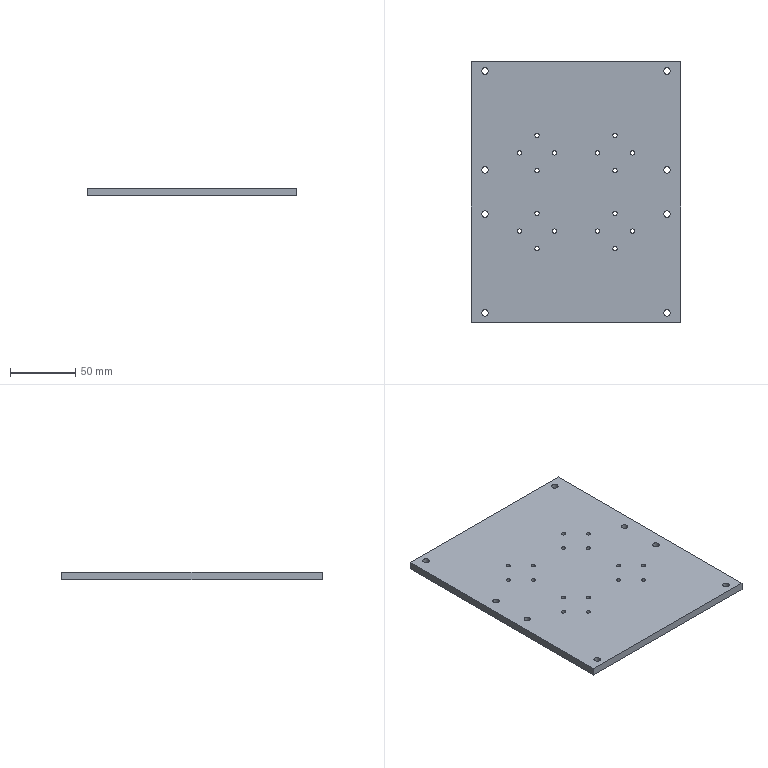Part | STEP file | Floating plate | 1 solid | 54 faces | box 161 x 200 x 6 mm | volume 191436 mm3 | cylinder 48 | plane 6 | commonest cylinder face diameters 3.3 x32 5 x16